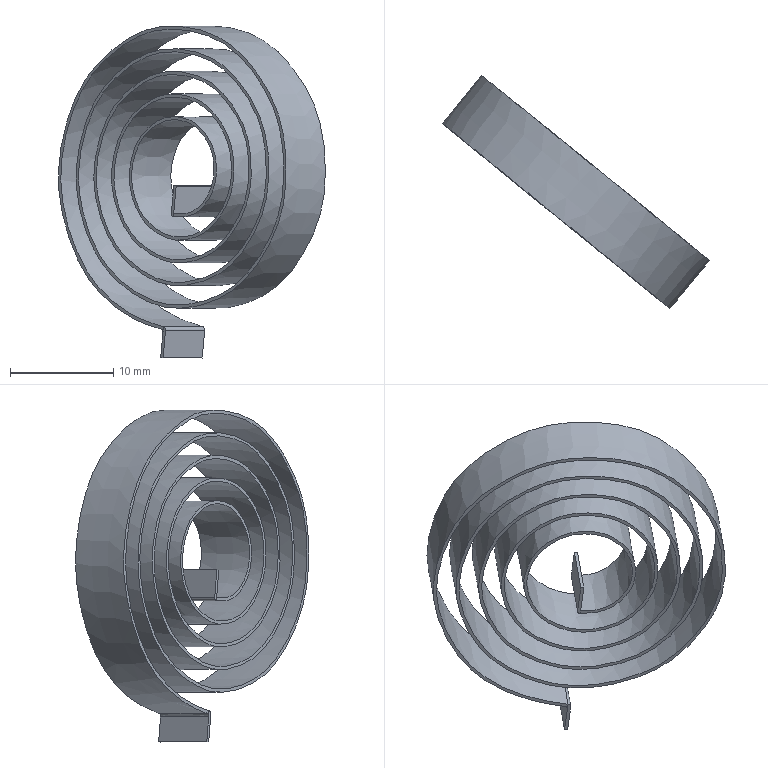Part | SolidWorks | features BaseBody 1 | 1 solid | 19 faces | box 25.833 x 22.578 x 32.112 mm | volume 551.538 mm3 | plane 11 | spline 5 | cylinder 3 | commonest cylinder face diameters 0.6 x3